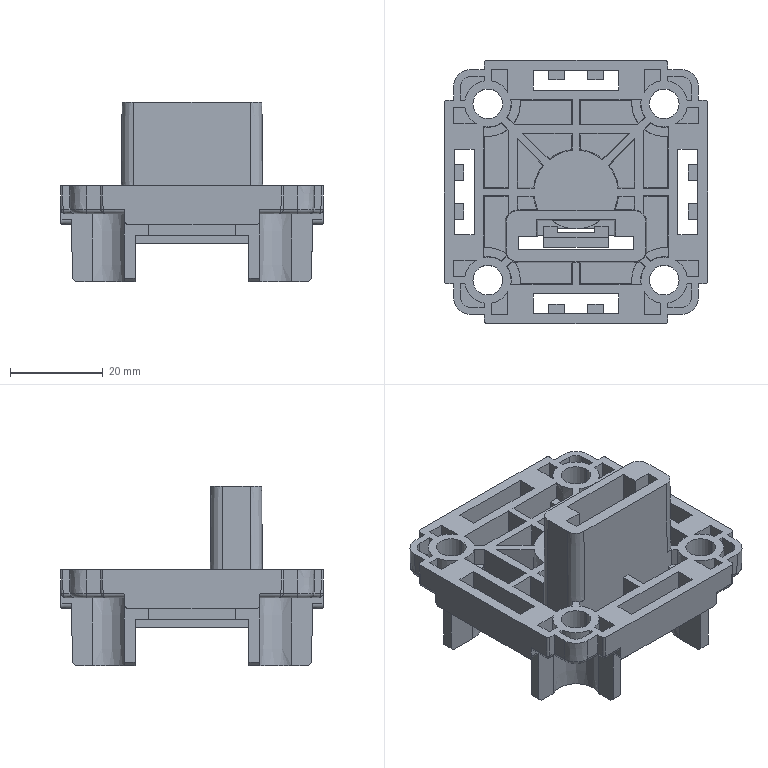Part | NX | features BREP 1 | 1 solid | 412 faces | box 56.75 x 56.75 x 38.616 mm | volume 22776 mm3 | plane 291 | cylinder 79 | cone 30 | spline 8 | torus 4 | commonest cylinder face diameters 2 x32 10 x12 1 x8 6.4 x8 14 x8 3 x4